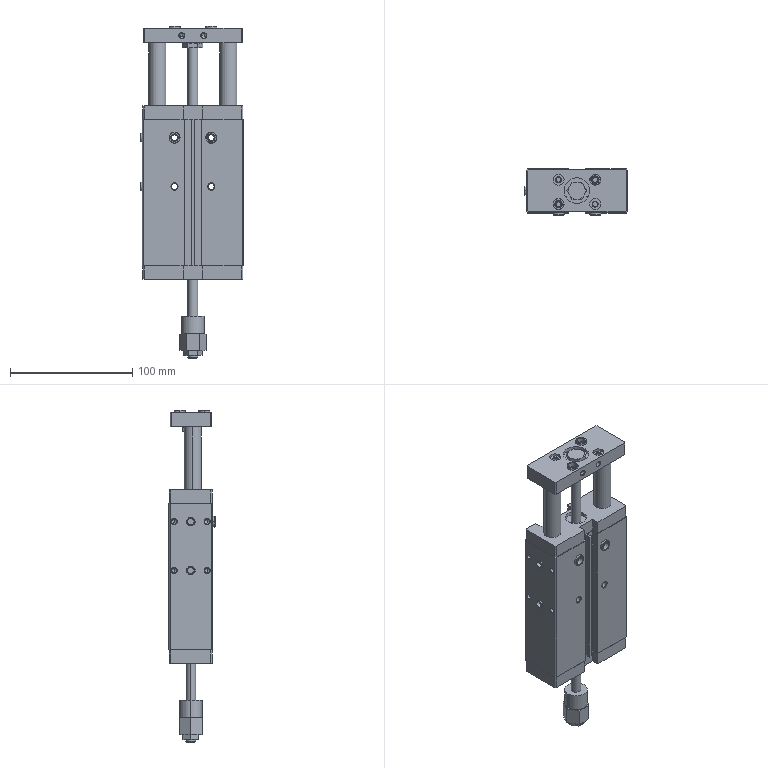Part | SolidWorks | 8 solids | 473 faces | box 84.4 x 37.9 x 271.9 mm | volume 422622 mm3 | plane 167 | cylinder 162 | cone 144 | commonest cylinder face diameters 4.134 x36 9 x28 0.4 x16 0.8 x14 5.3 x12 8 x10